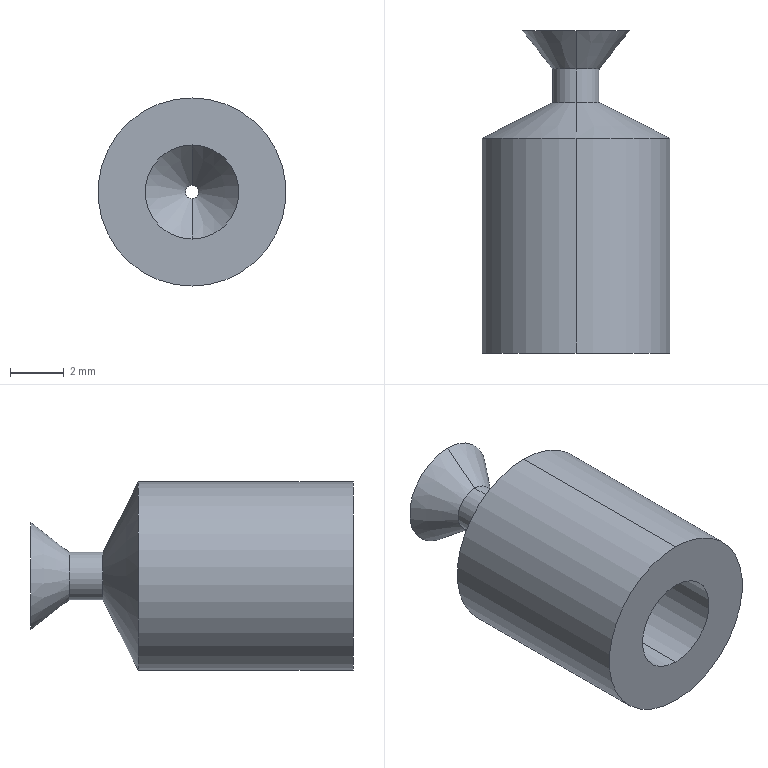Part | STEP file | ZP-04 | 1 solid | 18 faces | box 7 x 12 x 7 mm | volume 271.47 mm3 | cone 8 | cylinder 8 | plane 2 | commonest cylinder face diameters 0.5 x2 1.761 x2 3.5 x2 7 x2
STEP:
#1=CARTESIAN_POINT('',(0.,8.201,0.25));
#2=VERTEX_POINT('',#1);
#3=CARTESIAN_POINT('',(0.,8.201,-0.25));
#4=VERTEX_POINT('',#3);
#5=CARTESIAN_POINT('',(0.,8.201,0.));
#6=DIRECTION('',(0.,-1.,0.));
#7=DIRECTION('',(0.,0.,-1.));
#8=AXIS2_PLACEMENT_3D('',#5,#6,#7);
#9=CIRCLE('',#8,0.25);
#10=EDGE_CURVE('',#2,#4,#9,.T.);
#11=ORIENTED_EDGE('',*,*,#10,.F.);
#12=CARTESIAN_POINT('',(0.,6.568,1.75));
#13=VERTEX_POINT('',#12);
#14=CARTESIAN_POINT('',(0.,8.201,0.25));
#15=DIRECTION('',(0.,-0.7365,0.6765));
#16=VECTOR('',#15,1000.);
#17=LINE('',#14,#16);
#18=EDGE_CURVE('',#2,#13,#17,.T.);
#19=ORIENTED_EDGE('',*,*,#18,.T.);
#20=CARTESIAN_POINT('',(0.,6.568,-1.75));
#21=VERTEX_POINT('',#20);
#22=CARTESIAN_POINT('',(0.,6.568,0.));
#23=DIRECTION('',(0.,-1.,0.));
#24=DIRECTION('',(0.,0.,-1.));
#25=AXIS2_PLACEMENT_3D('',#22,#23,#24);
#26=CIRCLE('',#25,1.75);
#27=EDGE_CURVE('',#13,#21,#26,.T.);
#28=ORIENTED_EDGE('',*,*,#27,.T.);
#29=CARTESIAN_POINT('',(0.,8.201,-0.25));
#30=DIRECTION('',(0.,-0.7365,-0.6765));
#31=VECTOR('',#30,1000.);
#32=LINE('',#29,#31);
#33=EDGE_CURVE('',#4,#21,#32,.T.);
#34=ORIENTED_EDGE('',*,*,#33,.F.);
#35=EDGE_LOOP('',(#11,#19,#28,#34));
#36=FACE_OUTER_BOUND('',#35,.T.);
#37=CARTESIAN_POINT('',(0.,8.201,0.));
#38=DIRECTION('',(0.,-1.,0.));
#39=DIRECTION('',(0.,0.,-1.));
#40=AXIS2_PLACEMENT_3D('',#37,#38,#39);
#41=CONICAL_SURFACE('',#40,0.25,0.743);
#42=ADVANCED_FACE('',(#36),#41,.F.);
#43=CARTESIAN_POINT('',(0.,11.477,0.25));
#44=VERTEX_POINT('',#43);
#45=CARTESIAN_POINT('',(0.,11.477,-0.25));
#46=VERTEX_POINT('',#45);
#47=CARTESIAN_POINT('',(0.,11.477,0.));
#48=DIRECTION('',(0.,-1.,0.));
#49=DIRECTION('',(0.,0.,-1.));
#50=AXIS2_PLACEMENT_3D('',#47,#48,#49);
#51=CIRCLE('',#50,0.25);
#52=EDGE_CURVE('',#44,#46,#51,.T.);
#53=ORIENTED_EDGE('',*,*,#52,.F.);
#54=CARTESIAN_POINT('',(0.,0.,0.25));
#55=DIRECTION('',(0.,-1.,0.));
#56=VECTOR('',#55,1000.);
#57=LINE('',#54,#56);
#58=EDGE_CURVE('',#44,#2,#57,.T.);
#59=ORIENTED_EDGE('',*,*,#58,.T.);
#60=ORIENTED_EDGE('',*,*,#10,.T.);
#61=CARTESIAN_POINT('',(0.,0.,-0.25));
#62=DIRECTION('',(0.,-1.,0.));
#63=VECTOR('',#62,1000.);
#64=LINE('',#61,#63);
#65=EDGE_CURVE('',#46,#4,#64,.T.);
#66=ORIENTED_EDGE('',*,*,#65,.F.);
#67=EDGE_LOOP('',(#53,#59,#60,#66));
#68=FACE_OUTER_BOUND('',#67,.T.);
#69=CARTESIAN_POINT('',(0.,0.,0.));
#70=DIRECTION('',(0.,-1.,0.));
#71=DIRECTION('',(0.,0.,-1.));
#72=AXIS2_PLACEMENT_3D('',#69,#70,#71);
#73=CYLINDRICAL_SURFACE('',#72,0.25);
#74=ADVANCED_FACE('',(#68),#73,.F.);
#75=ORIENTED_EDGE('',*,*,#52,.T.);
#76=CARTESIAN_POINT('',(0.,12.,-1.541));
#77=VERTEX_POINT('',#76);
#78=CARTESIAN_POINT('',(0.,12.,-1.541));
#79=DIRECTION('',(0.,0.3755,-0.9268));
#80=VECTOR('',#79,1000.);
#81=LINE('',#78,#80);
#82=EDGE_CURVE('',#46,#77,#81,.T.);
#83=ORIENTED_EDGE('',*,*,#82,.T.);
#84=CARTESIAN_POINT('',(0.,12.,1.541));
#85=VERTEX_POINT('',#84);
#86=CARTESIAN_POINT('',(0.,12.,0.));
#87=DIRECTION('',(0.,-1.,0.));
#88=DIRECTION('',(0.,0.,-1.));
#89=AXIS2_PLACEMENT_3D('',#86,#87,#88);
#90=CIRCLE('',#89,1.541);
#91=EDGE_CURVE('',#85,#77,#90,.T.);
#92=ORIENTED_EDGE('',*,*,#91,.F.);
#93=CARTESIAN_POINT('',(0.,12.,1.541));
#94=DIRECTION('',(0.,0.3755,0.9268));
#95=VECTOR('',#94,1000.);
#96=LINE('',#93,#95);
#97=EDGE_CURVE('',#44,#85,#96,.T.);
#98=ORIENTED_EDGE('',*,*,#97,.F.);
#99=EDGE_LOOP('',(#75,#83,#92,#98));
#100=FACE_OUTER_BOUND('',#99,.T.);
#101=CARTESIAN_POINT('',(0.,12.,0.));
#102=DIRECTION('',(0.,1.,0.));
#103=DIRECTION('',(0.,0.,1.));
#104=AXIS2_PLACEMENT_3D('',#101,#102,#103);
#105=CONICAL_SURFACE('',#104,1.541,1.186);
#106=ADVANCED_FACE('',(#100),#105,.F.);
#107=CARTESIAN_POINT('',(0.,10.575,-0.8804));
#108=VERTEX_POINT('',#107);
#109=CARTESIAN_POINT('',(0.,10.575,0.8804));
#110=VERTEX_POINT('',#109);
#111=CARTESIAN_POINT('',(0.,10.575,0.));
#112=DIRECTION('',(0.,-1.,0.));
#113=DIRECTION('',(0.,0.,-1.));
#114=AXIS2_PLACEMENT_3D('',#111,#112,#113);
#115=CIRCLE('',#114,0.8804);
#116=EDGE_CURVE('',#108,#110,#115,.T.);
#117=ORIENTED_EDGE('',*,*,#116,.F.);
#118=CARTESIAN_POINT('',(0.,12.,-2.));
#119=VERTEX_POINT('',#118);
#120=CARTESIAN_POINT('',(0.,10.575,-0.8804));
#121=DIRECTION('',(0.,0.7863,-0.6178));
#122=VECTOR('',#121,1000.);
#123=LINE('',#120,#122);
#124=EDGE_CURVE('',#108,#119,#123,.T.);
#125=ORIENTED_EDGE('',*,*,#124,.T.);
#126=CARTESIAN_POINT('',(0.,12.,2.));
#127=VERTEX_POINT('',#126);
#128=CARTESIAN_POINT('',(0.,12.,0.));
#129=DIRECTION('',(0.,-1.,0.));
#130=DIRECTION('',(0.,0.,-1.));
#131=AXIS2_PLACEMENT_3D('',#128,#129,#130);
#132=CIRCLE('',#131,2.);
#133=EDGE_CURVE('',#119,#127,#132,.T.);
#134=ORIENTED_EDGE('',*,*,#133,.T.);
#135=CARTESIAN_POINT('',(0.,10.575,0.8804));
#136=DIRECTION('',(0.,0.7863,0.6178));
#137=VECTOR('',#136,1000.);
#138=LINE('',#135,#137);
#139=EDGE_CURVE('',#110,#127,#138,.T.);
#140=ORIENTED_EDGE('',*,*,#139,.F.);
#141=EDGE_LOOP('',(#117,#125,#134,#140));
#142=FACE_OUTER_BOUND('',#141,.T.);
#143=CARTESIAN_POINT('',(0.,10.575,0.));
#144=DIRECTION('',(0.,1.,0.));
#145=DIRECTION('',(0.,0.,1.));
#146=AXIS2_PLACEMENT_3D('',#143,#144,#145);
#147=CONICAL_SURFACE('',#146,0.8804,0.666);
#148=ADVANCED_FACE('',(#142),#147,.T.);
#149=ORIENTED_EDGE('',*,*,#116,.T.);
#150=CARTESIAN_POINT('',(0.,9.32,0.8804));
#151=VERTEX_POINT('',#150);
#152=CARTESIAN_POINT('',(0.,0.,0.8804));
#153=DIRECTION('',(0.,-1.,0.));
#154=VECTOR('',#153,1000.);
#155=LINE('',#152,#154);
#156=EDGE_CURVE('',#110,#151,#155,.T.);
#157=ORIENTED_EDGE('',*,*,#156,.T.);
#158=CARTESIAN_POINT('',(0.,9.32,-0.8804));
#159=VERTEX_POINT('',#158);
#160=CARTESIAN_POINT('',(0.,9.32,0.));
#161=DIRECTION('',(0.,-1.,0.));
#162=DIRECTION('',(0.,0.,-1.));
#163=AXIS2_PLACEMENT_3D('',#160,#161,#162);
#164=CIRCLE('',#163,0.8804);
#165=EDGE_CURVE('',#159,#151,#164,.T.);
#166=ORIENTED_EDGE('',*,*,#165,.F.);
#167=CARTESIAN_POINT('',(0.,0.,-0.8804));
#168=DIRECTION('',(0.,-1.,0.));
#169=VECTOR('',#168,1000.);
#170=LINE('',#167,#169);
#171=EDGE_CURVE('',#108,#159,#170,.T.);
#172=ORIENTED_EDGE('',*,*,#171,.F.);
#173=EDGE_LOOP('',(#149,#157,#166,#172));
#174=FACE_OUTER_BOUND('',#173,.T.);
#175=CARTESIAN_POINT('',(0.,0.,0.));
#176=DIRECTION('',(0.,-1.,0.));
#177=DIRECTION('',(0.,0.,-1.));
#178=AXIS2_PLACEMENT_3D('',#175,#176,#177);
#179=CYLINDRICAL_SURFACE('',#178,0.8804);
#180=ADVANCED_FACE('',(#174),#179,.T.);
#181=ORIENTED_EDGE('',*,*,#165,.T.);
#182=CARTESIAN_POINT('',(0.,8.,3.5));
#183=VERTEX_POINT('',#182);
#184=CARTESIAN_POINT('',(0.,8.,3.5));
#185=DIRECTION('',(0.,-0.45,0.893));
#186=VECTOR('',#185,1000.);
#187=LINE('',#184,#186);
#188=EDGE_CURVE('',#151,#183,#187,.T.);
#189=ORIENTED_EDGE('',*,*,#188,.T.);
#190=CARTESIAN_POINT('',(0.,8.,-3.5));
#191=VERTEX_POINT('',#190);
#192=CARTESIAN_POINT('',(0.,8.,0.));
#193=DIRECTION('',(0.,-1.,0.));
#194=DIRECTION('',(0.,0.,-1.));
#195=AXIS2_PLACEMENT_3D('',#192,#193,#194);
#196=CIRCLE('',#195,3.5);
#197=EDGE_CURVE('',#191,#183,#196,.T.);
#198=ORIENTED_EDGE('',*,*,#197,.F.);
#199=CARTESIAN_POINT('',(0.,8.,-3.5));
#200=DIRECTION('',(0.,-0.45,-0.893));
#201=VECTOR('',#200,1000.);
#202=LINE('',#199,#201);
#203=EDGE_CURVE('',#159,#191,#202,.T.);
#204=ORIENTED_EDGE('',*,*,#203,.F.);
#205=EDGE_LOOP('',(#181,#189,#198,#204));
#206=FACE_OUTER_BOUND('',#205,.T.);
#207=CARTESIAN_POINT('',(0.,8.,0.));
#208=DIRECTION('',(0.,-1.,0.));
#209=DIRECTION('',(0.,0.,-1.));
#210=AXIS2_PLACEMENT_3D('',#207,#208,#209);
#211=CONICAL_SURFACE('',#210,3.5,1.104);
#212=ADVANCED_FACE('',(#206),#211,.T.);
#213=ORIENTED_EDGE('',*,*,#197,.T.);
#214=CARTESIAN_POINT('',(0.,0.,3.5));
#215=VERTEX_POINT('',#214);
#216=CARTESIAN_POINT('',(0.,0.,3.5));
#217=DIRECTION('',(0.,-1.,0.));
#218=VECTOR('',#217,1000.);
#219=LINE('',#216,#218);
#220=EDGE_CURVE('',#183,#215,#219,.T.);
#221=ORIENTED_EDGE('',*,*,#220,.T.);
#222=CARTESIAN_POINT('',(0.,0.,-3.5));
#223=VERTEX_POINT('',#222);
#224=CARTESIAN_POINT('',(0.,0.,0.));
#225=DIRECTION('',(0.,-1.,0.));
#226=DIRECTION('',(0.,0.,-1.));
#227=AXIS2_PLACEMENT_3D('',#224,#225,#226);
#228=CIRCLE('',#227,3.5);
#229=EDGE_CURVE('',#223,#215,#228,.T.);
#230=ORIENTED_EDGE('',*,*,#229,.F.);
#231=CARTESIAN_POINT('',(0.,0.,-3.5));
#232=DIRECTION('',(0.,-1.,0.));
#233=VECTOR('',#232,1000.);
#234=LINE('',#231,#233);
#235=EDGE_CURVE('',#191,#223,#234,.T.);
#236=ORIENTED_EDGE('',*,*,#235,.F.);
#237=EDGE_LOOP('',(#213,#221,#230,#236));
#238=FACE_OUTER_BOUND('',#237,.T.);
#239=CARTESIAN_POINT('',(0.,0.,0.));
#240=DIRECTION('',(0.,-1.,0.));
#241=DIRECTION('',(0.,0.,-1.));
#242=AXIS2_PLACEMENT_3D('',#239,#240,#241);
#243=CYLINDRICAL_SURFACE('',#242,3.5);
#244=ADVANCED_FACE('',(#238),#243,.T.);
#245=ORIENTED_EDGE('',*,*,#27,.F.);
#246=CARTESIAN_POINT('',(0.,0.,1.75));
#247=VERTEX_POINT('',#246);
#248=CARTESIAN_POINT('',(0.,0.,1.75));
#249=DIRECTION('',(0.,-1.,0.));
#250=VECTOR('',#249,1000.);
#251=LINE('',#248,#250);
#252=EDGE_CURVE('',#13,#247,#251,.T.);
#253=ORIENTED_EDGE('',*,*,#252,.T.);
#254=CARTESIAN_POINT('',(0.,0.,-1.75));
#255=VERTEX_POINT('',#254);
#256=CARTESIAN_POINT('',(0.,0.,0.));
#257=DIRECTION('',(0.,-1.,0.));
#258=DIRECTION('',(0.,0.,-1.));
#259=AXIS2_PLACEMENT_3D('',#256,#257,#258);
#260=CIRCLE('',#259,1.75);
#261=EDGE_CURVE('',#247,#255,#260,.T.);
#262=ORIENTED_EDGE('',*,*,#261,.T.);
#263=CARTESIAN_POINT('',(0.,0.,-1.75));
#264=DIRECTION('',(0.,-1.,0.));
#265=VECTOR('',#264,1000.);
#266=LINE('',#263,#265);
#267=EDGE_CURVE('',#21,#255,#266,.T.);
#268=ORIENTED_EDGE('',*,*,#267,.F.);
#269=EDGE_LOOP('',(#245,#253,#262,#268));
#270=FACE_OUTER_BOUND('',#269,.T.);
#271=CARTESIAN_POINT('',(0.,0.,0.));
#272=DIRECTION('',(0.,-1.,0.));
#273=DIRECTION('',(0.,0.,-1.));
#274=AXIS2_PLACEMENT_3D('',#271,#272,#273);
#275=CYLINDRICAL_SURFACE('',#274,1.75);
#276=ADVANCED_FACE('',(#270),#275,.F.);
#277=ORIENTED_EDGE('',*,*,#252,.F.);
#278=CARTESIAN_POINT('',(0.,6.568,0.));
#279=DIRECTION('',(0.,-1.,0.));
#280=DIRECTION('',(0.,0.,-1.));
#281=AXIS2_PLACEMENT_3D('',#278,#279,#280);
#282=CIRCLE('',#281,1.75);
#283=EDGE_CURVE('',#21,#13,#282,.T.);
#284=ORIENTED_EDGE('',*,*,#283,.F.);
#285=ORIENTED_EDGE('',*,*,#267,.T.);
#286=CARTESIAN_POINT('',(0.,0.,0.));
#287=DIRECTION('',(0.,-1.,0.));
#288=DIRECTION('',(0.,0.,-1.));
#289=AXIS2_PLACEMENT_3D('',#286,#287,#288);
#290=CIRCLE('',#289,1.75);
#291=EDGE_CURVE('',#255,#247,#290,.T.);
#292=ORIENTED_EDGE('',*,*,#291,.T.);
#293=EDGE_LOOP('',(#277,#284,#285,#292));
#294=FACE_OUTER_BOUND('',#293,.T.);
#295=CARTESIAN_POINT('',(0.,0.,0.));
#296=DIRECTION('',(0.,-1.,0.));
#297=DIRECTION('',(0.,0.,-1.));
#298=AXIS2_PLACEMENT_3D('',#295,#296,#297);
#299=CYLINDRICAL_SURFACE('',#298,1.75);
#300=ADVANCED_FACE('',(#294),#299,.F.);
#301=ORIENTED_EDGE('',*,*,#229,.T.);
#302=CARTESIAN_POINT('',(0.,0.,0.));
#303=DIRECTION('',(0.,-1.,0.));
#304=DIRECTION('',(0.,0.,-1.));
#305=AXIS2_PLACEMENT_3D('',#302,#303,#304);
#306=CIRCLE('',#305,3.5);
#307=EDGE_CURVE('',#215,#223,#306,.T.);
#308=ORIENTED_EDGE('',*,*,#307,.T.);
#309=EDGE_LOOP('',(#301,#308));
#310=FACE_OUTER_BOUND('',#309,.T.);
#311=ORIENTED_EDGE('',*,*,#291,.F.);
#312=ORIENTED_EDGE('',*,*,#261,.F.);
#313=EDGE_LOOP('',(#311,#312));
#314=FACE_BOUND('',#313,.T.);
#315=CARTESIAN_POINT('',(1.75,0.,0.));
#316=DIRECTION('',(0.,-1.,0.));
#317=DIRECTION('',(0.,0.,-1.));
#318=AXIS2_PLACEMENT_3D('',#315,#316,#317);
#319=PLANE('',#318);
#320=ADVANCED_FACE('',(#310,#314),#319,.T.);
#321=ORIENTED_EDGE('',*,*,#220,.F.);
#322=CARTESIAN_POINT('',(0.,8.,0.));
#323=DIRECTION('',(0.,-1.,0.));
#324=DIRECTION('',(0.,0.,-1.));
#325=AXIS2_PLACEMENT_3D('',#322,#323,#324);
#326=CIRCLE('',#325,3.5);
#327=EDGE_CURVE('',#183,#191,#326,.T.);
#328=ORIENTED_EDGE('',*,*,#327,.T.);
#329=ORIENTED_EDGE('',*,*,#235,.T.);
#330=ORIENTED_EDGE('',*,*,#307,.F.);
#331=EDGE_LOOP('',(#321,#328,#329,#330));
#332=FACE_OUTER_BOUND('',#331,.T.);
#333=CARTESIAN_POINT('',(0.,0.,0.));
#334=DIRECTION('',(0.,-1.,0.));
#335=DIRECTION('',(0.,0.,-1.));
#336=AXIS2_PLACEMENT_3D('',#333,#334,#335);
#337=CYLINDRICAL_SURFACE('',#336,3.5);
#338=ADVANCED_FACE('',(#332),#337,.T.);
#339=ORIENTED_EDGE('',*,*,#188,.F.);
#340=CARTESIAN_POINT('',(0.,9.32,0.));
#341=DIRECTION('',(0.,-1.,0.));
#342=DIRECTION('',(0.,0.,-1.));
#343=AXIS2_PLACEMENT_3D('',#340,#341,#342);
#344=CIRCLE('',#343,0.8804);
#345=EDGE_CURVE('',#151,#159,#344,.T.);
#346=ORIENTED_EDGE('',*,*,#345,.T.);
#347=ORIENTED_EDGE('',*,*,#203,.T.);
#348=ORIENTED_EDGE('',*,*,#327,.F.);
#349=EDGE_LOOP('',(#339,#346,#347,#348));
#350=FACE_OUTER_BOUND('',#349,.T.);
#351=CARTESIAN_POINT('',(0.,8.,0.));
#352=DIRECTION('',(0.,-1.,0.));
#353=DIRECTION('',(0.,0.,-1.));
#354=AXIS2_PLACEMENT_3D('',#351,#352,#353);
#355=CONICAL_SURFACE('',#354,3.5,1.104);
#356=ADVANCED_FACE('',(#350),#355,.T.);
#357=ORIENTED_EDGE('',*,*,#156,.F.);
#358=CARTESIAN_POINT('',(0.,10.575,0.));
#359=DIRECTION('',(0.,-1.,0.));
#360=DIRECTION('',(0.,0.,-1.));
#361=AXIS2_PLACEMENT_3D('',#358,#359,#360);
#362=CIRCLE('',#361,0.8804);
#363=EDGE_CURVE('',#110,#108,#362,.T.);
#364=ORIENTED_EDGE('',*,*,#363,.T.);
#365=ORIENTED_EDGE('',*,*,#171,.T.);
#366=ORIENTED_EDGE('',*,*,#345,.F.);
#367=EDGE_LOOP('',(#357,#364,#365,#366));
#368=FACE_OUTER_BOUND('',#367,.T.);
#369=CARTESIAN_POINT('',(0.,0.,0.));
#370=DIRECTION('',(0.,-1.,0.));
#371=DIRECTION('',(0.,0.,-1.));
#372=AXIS2_PLACEMENT_3D('',#369,#370,#371);
#373=CYLINDRICAL_SURFACE('',#372,0.8804);
#374=ADVANCED_FACE('',(#368),#373,.T.);
#375=ORIENTED_EDGE('',*,*,#124,.F.);
#376=ORIENTED_EDGE('',*,*,#363,.F.);
#377=ORIENTED_EDGE('',*,*,#139,.T.);
#378=CARTESIAN_POINT('',(0.,12.,0.));
#379=DIRECTION('',(0.,-1.,0.));
#380=DIRECTION('',(0.,0.,-1.));
#381=AXIS2_PLACEMENT_3D('',#378,#379,#380);
#382=CIRCLE('',#381,2.);
#383=EDGE_CURVE('',#127,#119,#382,.T.);
#384=ORIENTED_EDGE('',*,*,#383,.T.);
#385=EDGE_LOOP('',(#375,#376,#377,#384));
#386=FACE_OUTER_BOUND('',#385,.T.);
#387=CARTESIAN_POINT('',(0.,10.575,0.));
#388=DIRECTION('',(0.,1.,0.));
#389=DIRECTION('',(0.,0.,1.));
#390=AXIS2_PLACEMENT_3D('',#387,#388,#389);
#391=CONICAL_SURFACE('',#390,0.8804,0.666);
#392=ADVANCED_FACE('',(#386),#391,.T.);
#393=ORIENTED_EDGE('',*,*,#91,.T.);
#394=CARTESIAN_POINT('',(0.,12.,0.));
#395=DIRECTION('',(0.,-1.,0.));
#396=DIRECTION('',(0.,0.,-1.));
#397=AXIS2_PLACEMENT_3D('',#394,#395,#396);
#398=CIRCLE('',#397,1.541);
#399=EDGE_CURVE('',#77,#85,#398,.T.);
#400=ORIENTED_EDGE('',*,*,#399,.T.);
#401=EDGE_LOOP('',(#393,#400));
#402=FACE_BOUND('',#401,.T.);
#403=ORIENTED_EDGE('',*,*,#383,.F.);
#404=ORIENTED_EDGE('',*,*,#133,.F.);
#405=EDGE_LOOP('',(#403,#404));
#406=FACE_OUTER_BOUND('',#405,.T.);
#407=CARTESIAN_POINT('',(2.,12.,0.));
#408=DIRECTION('',(0.,1.,0.));
#409=DIRECTION('',(0.,0.,1.));
#410=AXIS2_PLACEMENT_3D('',#407,#408,#409);
#411=PLANE('',#410);
#412=ADVANCED_FACE('',(#402,#406),#411,.T.);
#413=ORIENTED_EDGE('',*,*,#82,.F.);
#414=CARTESIAN_POINT('',(0.,11.477,0.));
#415=DIRECTION('',(0.,-1.,0.));
#416=DIRECTION('',(0.,0.,-1.));
#417=AXIS2_PLACEMENT_3D('',#414,#415,#416);
#418=CIRCLE('',#417,0.25);
#419=EDGE_CURVE('',#46,#44,#418,.T.);
#420=ORIENTED_EDGE('',*,*,#419,.T.);
#421=ORIENTED_EDGE('',*,*,#97,.T.);
#422=ORIENTED_EDGE('',*,*,#399,.F.);
#423=EDGE_LOOP('',(#413,#420,#421,#422));
#424=FACE_OUTER_BOUND('',#423,.T.);
#425=CARTESIAN_POINT('',(0.,12.,0.));
#426=DIRECTION('',(0.,1.,0.));
#427=DIRECTION('',(0.,0.,1.));
#428=AXIS2_PLACEMENT_3D('',#425,#426,#427);
#429=CONICAL_SURFACE('',#428,1.541,1.186);
#430=ADVANCED_FACE('',(#424),#429,.F.);
#431=ORIENTED_EDGE('',*,*,#58,.F.);
#432=ORIENTED_EDGE('',*,*,#419,.F.);
#433=ORIENTED_EDGE('',*,*,#65,.T.);
#434=CARTESIAN_POINT('',(0.,8.201,0.));
#435=DIRECTION('',(0.,-1.,0.));
#436=DIRECTION('',(0.,0.,-1.));
#437=AXIS2_PLACEMENT_3D('',#434,#435,#436);
#438=CIRCLE('',#437,0.25);
#439=EDGE_CURVE('',#4,#2,#438,.T.);
#440=ORIENTED_EDGE('',*,*,#439,.T.);
#441=EDGE_LOOP('',(#431,#432,#433,#440));
#442=FACE_OUTER_BOUND('',#441,.T.);
#443=CARTESIAN_POINT('',(0.,0.,0.));
#444=DIRECTION('',(0.,-1.,0.));
#445=DIRECTION('',(0.,0.,-1.));
#446=AXIS2_PLACEMENT_3D('',#443,#444,#445);
#447=CYLINDRICAL_SURFACE('',#446,0.25);
#448=ADVANCED_FACE('',(#442),#447,.F.);
#449=ORIENTED_EDGE('',*,*,#18,.F.);
#450=ORIENTED_EDGE('',*,*,#439,.F.);
#451=ORIENTED_EDGE('',*,*,#33,.T.);
#452=ORIENTED_EDGE('',*,*,#283,.T.);
#453=EDGE_LOOP('',(#449,#450,#451,#452));
#454=FACE_OUTER_BOUND('',#453,.T.);
#455=CARTESIAN_POINT('',(0.,8.201,0.));
#456=DIRECTION('',(0.,-1.,0.));
#457=DIRECTION('',(0.,0.,-1.));
#458=AXIS2_PLACEMENT_3D('',#455,#456,#457);
#459=CONICAL_SURFACE('',#458,0.25,0.743);
#460=ADVANCED_FACE('',(#454),#459,.F.);
#461=CLOSED_SHELL('',(#42,#74,#106,#148,#180,#212,#244,#276,#300,#320,#338,#356,#374,#392,#412,#430,#448,#460));
#462=MANIFOLD_SOLID_BREP('',#461);
#463=CARTESIAN_POINT('',(0.,0.,0.));
#464=DIRECTION('',(0.,0.,1.));
#465=DIRECTION('',(1.,0.,0.));
#466=AXIS2_PLACEMENT_3D('',#463,#464,#465);
#467=(LENGTH_UNIT()NAMED_UNIT(*)SI_UNIT(.MILLI.,.METRE.));
#468=UNCERTAINTY_MEASURE_WITH_UNIT(LENGTH_MEASURE(0.00001),#467,'','');
#469=(NAMED_UNIT(*)PLANE_ANGLE_UNIT()SI_UNIT($,.RADIAN.));
#470=(NAMED_UNIT(*)SI_UNIT($,.STERADIAN.)SOLID_ANGLE_UNIT());
#471=(GEOMETRIC_REPRESENTATION_CONTEXT(3)GLOBAL_UNCERTAINTY_ASSIGNED_CONTEXT((#468))GLOBAL_UNIT_ASSIGNED_CONTEXT((#467,#469,#470))REPRESENTATION_CONTEXT('',''));
#472=ADVANCED_BREP_SHAPE_REPRESENTATION('',(#462,#466),#471);